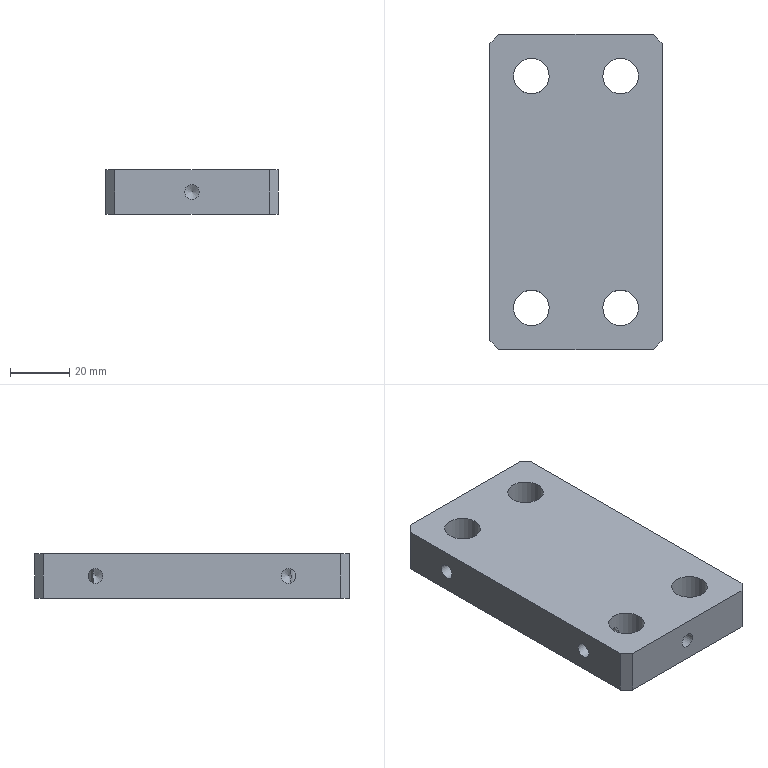Part | NX | features BREP 1 | 1 solid | 20 faces | box 58 x 106 x 15 mm | volume 84312 mm3 | plane 10 | cylinder 7 | cone 3 | commonest cylinder face diameters 12 x4 5 x3
STEP:
#1=CARTESIAN_POINT('',(-29.,50.,15.));
#2=VERTEX_POINT('',#1);
#3=CARTESIAN_POINT('',(-29.,-50.,15.));
#4=VERTEX_POINT('',#3);
#5=CARTESIAN_POINT('',(-29.,0.,15.));
#6=DIRECTION('',(0.,-1.,0.));
#7=VECTOR('',#6,1000.);
#8=LINE('',#5,#7);
#9=EDGE_CURVE('',#2,#4,#8,.T.);
#10=ORIENTED_EDGE('',*,*,#9,.T.);
#11=CARTESIAN_POINT('',(-26.,-53.,15.));
#12=VERTEX_POINT('',#11);
#13=CARTESIAN_POINT('',(-29.,-50.,15.));
#14=DIRECTION('',(0.7071,-0.7071,0.));
#15=VECTOR('',#14,1000.);
#16=LINE('',#13,#15);
#17=EDGE_CURVE('',#4,#12,#16,.T.);
#18=ORIENTED_EDGE('',*,*,#17,.T.);
#19=CARTESIAN_POINT('',(26.,-53.,15.));
#20=VERTEX_POINT('',#19);
#21=CARTESIAN_POINT('',(0.,-53.,15.));
#22=DIRECTION('',(1.,0.,0.));
#23=VECTOR('',#22,1000.);
#24=LINE('',#21,#23);
#25=EDGE_CURVE('',#12,#20,#24,.T.);
#26=ORIENTED_EDGE('',*,*,#25,.T.);
#27=CARTESIAN_POINT('',(29.,-50.,15.));
#28=VERTEX_POINT('',#27);
#29=CARTESIAN_POINT('',(26.,-53.,15.));
#30=DIRECTION('',(0.7071,0.7071,0.));
#31=VECTOR('',#30,1000.);
#32=LINE('',#29,#31);
#33=EDGE_CURVE('',#20,#28,#32,.T.);
#34=ORIENTED_EDGE('',*,*,#33,.T.);
#35=CARTESIAN_POINT('',(29.,50.,15.));
#36=VERTEX_POINT('',#35);
#37=CARTESIAN_POINT('',(29.,0.,15.));
#38=DIRECTION('',(0.,1.,0.));
#39=VECTOR('',#38,1000.);
#40=LINE('',#37,#39);
#41=EDGE_CURVE('',#28,#36,#40,.T.);
#42=ORIENTED_EDGE('',*,*,#41,.T.);
#43=CARTESIAN_POINT('',(26.,53.,15.));
#44=VERTEX_POINT('',#43);
#45=CARTESIAN_POINT('',(29.,50.,15.));
#46=DIRECTION('',(-0.7071,0.7071,0.));
#47=VECTOR('',#46,1000.);
#48=LINE('',#45,#47);
#49=EDGE_CURVE('',#36,#44,#48,.T.);
#50=ORIENTED_EDGE('',*,*,#49,.T.);
#51=CARTESIAN_POINT('',(-26.,53.,15.));
#52=VERTEX_POINT('',#51);
#53=CARTESIAN_POINT('',(0.,53.,15.));
#54=DIRECTION('',(-1.,0.,0.));
#55=VECTOR('',#54,1000.);
#56=LINE('',#53,#55);
#57=EDGE_CURVE('',#44,#52,#56,.T.);
#58=ORIENTED_EDGE('',*,*,#57,.T.);
#59=CARTESIAN_POINT('',(-26.,53.,15.));
#60=DIRECTION('',(-0.7071,-0.7071,0.));
#61=VECTOR('',#60,1000.);
#62=LINE('',#59,#61);
#63=EDGE_CURVE('',#52,#2,#62,.T.);
#64=ORIENTED_EDGE('',*,*,#63,.T.);
#65=EDGE_LOOP('',(#10,#18,#26,#34,#42,#50,#58,#64));
#66=FACE_BOUND('',#65,.T.);
#67=CARTESIAN_POINT('',(9.,-39.,15.));
#68=VERTEX_POINT('',#67);
#69=CARTESIAN_POINT('',(15.,-39.,15.));
#70=DIRECTION('',(0.,0.,-1.));
#71=DIRECTION('',(-1.,0.,0.));
#72=AXIS2_PLACEMENT_3D('',#69,#70,#71);
#73=CIRCLE('',#72,6.);
#74=EDGE_CURVE('',#68,#68,#73,.T.);
#75=ORIENTED_EDGE('',*,*,#74,.T.);
#76=EDGE_LOOP('',(#75));
#77=FACE_BOUND('',#76,.T.);
#78=CARTESIAN_POINT('',(-21.,-39.,15.));
#79=VERTEX_POINT('',#78);
#80=CARTESIAN_POINT('',(-15.,-39.,15.));
#81=DIRECTION('',(0.,0.,-1.));
#82=DIRECTION('',(-1.,0.,0.));
#83=AXIS2_PLACEMENT_3D('',#80,#81,#82);
#84=CIRCLE('',#83,6.);
#85=EDGE_CURVE('',#79,#79,#84,.T.);
#86=ORIENTED_EDGE('',*,*,#85,.T.);
#87=EDGE_LOOP('',(#86));
#88=FACE_BOUND('',#87,.T.);
#89=CARTESIAN_POINT('',(-21.,39.,15.));
#90=VERTEX_POINT('',#89);
#91=CARTESIAN_POINT('',(-15.,39.,15.));
#92=DIRECTION('',(0.,0.,-1.));
#93=DIRECTION('',(-1.,0.,0.));
#94=AXIS2_PLACEMENT_3D('',#91,#92,#93);
#95=CIRCLE('',#94,6.);
#96=EDGE_CURVE('',#90,#90,#95,.T.);
#97=ORIENTED_EDGE('',*,*,#96,.T.);
#98=EDGE_LOOP('',(#97));
#99=FACE_BOUND('',#98,.T.);
#100=CARTESIAN_POINT('',(9.,39.,15.));
#101=VERTEX_POINT('',#100);
#102=CARTESIAN_POINT('',(15.,39.,15.));
#103=DIRECTION('',(0.,0.,-1.));
#104=DIRECTION('',(-1.,0.,0.));
#105=AXIS2_PLACEMENT_3D('',#102,#103,#104);
#106=CIRCLE('',#105,6.);
#107=EDGE_CURVE('',#101,#101,#106,.T.);
#108=ORIENTED_EDGE('',*,*,#107,.T.);
#109=EDGE_LOOP('',(#108));
#110=FACE_BOUND('',#109,.T.);
#111=CARTESIAN_POINT('',(0.,0.,15.));
#112=DIRECTION('',(0.,0.,1.));
#113=DIRECTION('',(-1.,0.,0.));
#114=AXIS2_PLACEMENT_3D('',#111,#112,#113);
#115=PLANE('',#114);
#116=ADVANCED_FACE('',(#66,#77,#88,#99,#110),#115,.T.);
#117=CARTESIAN_POINT('',(-29.,-50.,0.));
#118=VERTEX_POINT('',#117);
#119=CARTESIAN_POINT('',(-29.,-50.,15.));
#120=DIRECTION('',(0.,0.,1.));
#121=VECTOR('',#120,1000.);
#122=LINE('',#119,#121);
#123=EDGE_CURVE('',#118,#4,#122,.T.);
#124=ORIENTED_EDGE('',*,*,#123,.F.);
#125=CARTESIAN_POINT('',(-26.,-53.,0.));
#126=VERTEX_POINT('',#125);
#127=CARTESIAN_POINT('',(-26.,-53.,0.));
#128=DIRECTION('',(-0.7071,0.7071,0.));
#129=VECTOR('',#128,1000.);
#130=LINE('',#127,#129);
#131=EDGE_CURVE('',#126,#118,#130,.T.);
#132=ORIENTED_EDGE('',*,*,#131,.F.);
#133=CARTESIAN_POINT('',(-26.,-53.,15.));
#134=DIRECTION('',(0.,0.,-1.));
#135=VECTOR('',#134,1000.);
#136=LINE('',#133,#135);
#137=EDGE_CURVE('',#12,#126,#136,.T.);
#138=ORIENTED_EDGE('',*,*,#137,.F.);
#139=ORIENTED_EDGE('',*,*,#17,.F.);
#140=EDGE_LOOP('',(#124,#132,#138,#139));
#141=FACE_BOUND('',#140,.T.);
#142=CARTESIAN_POINT('',(-26.,-53.,15.));
#143=DIRECTION('',(0.7071,0.7071,0.));
#144=DIRECTION('',(0.7071,-0.7071,0.));
#145=AXIS2_PLACEMENT_3D('',#142,#143,#144);
#146=PLANE('',#145);
#147=ADVANCED_FACE('',(#141),#146,.F.);
#148=ORIENTED_EDGE('',*,*,#123,.T.);
#149=ORIENTED_EDGE('',*,*,#9,.F.);
#150=CARTESIAN_POINT('',(-29.,50.,0.));
#151=VERTEX_POINT('',#150);
#152=CARTESIAN_POINT('',(-29.,50.,15.));
#153=DIRECTION('',(0.,0.,1.));
#154=VECTOR('',#153,1000.);
#155=LINE('',#152,#154);
#156=EDGE_CURVE('',#151,#2,#155,.T.);
#157=ORIENTED_EDGE('',*,*,#156,.F.);
#158=CARTESIAN_POINT('',(-29.,53.,0.));
#159=DIRECTION('',(0.,1.,0.));
#160=VECTOR('',#159,1000.);
#161=LINE('',#158,#160);
#162=EDGE_CURVE('',#118,#151,#161,.T.);
#163=ORIENTED_EDGE('',*,*,#162,.F.);
#164=EDGE_LOOP('',(#148,#149,#157,#163));
#165=FACE_BOUND('',#164,.T.);
#166=CARTESIAN_POINT('',(-29.,32.5,10.));
#167=VERTEX_POINT('',#166);
#168=CARTESIAN_POINT('',(-29.,32.5,7.5));
#169=DIRECTION('',(-1.,0.,0.));
#170=DIRECTION('',(0.,0.,1.));
#171=AXIS2_PLACEMENT_3D('',#168,#169,#170);
#172=CIRCLE('',#171,2.5);
#173=EDGE_CURVE('',#167,#167,#172,.T.);
#174=ORIENTED_EDGE('',*,*,#173,.F.);
#175=EDGE_LOOP('',(#174));
#176=FACE_BOUND('',#175,.T.);
#177=CARTESIAN_POINT('',(-29.,-32.5,10.));
#178=VERTEX_POINT('',#177);
#179=CARTESIAN_POINT('',(-29.,-32.5,7.5));
#180=DIRECTION('',(-1.,0.,0.));
#181=DIRECTION('',(0.,0.,1.));
#182=AXIS2_PLACEMENT_3D('',#179,#180,#181);
#183=CIRCLE('',#182,2.5);
#184=EDGE_CURVE('',#178,#178,#183,.T.);
#185=ORIENTED_EDGE('',*,*,#184,.F.);
#186=EDGE_LOOP('',(#185));
#187=FACE_BOUND('',#186,.T.);
#188=CARTESIAN_POINT('',(-29.,53.,15.));
#189=DIRECTION('',(1.,0.,0.));
#190=DIRECTION('',(0.,-1.,0.));
#191=AXIS2_PLACEMENT_3D('',#188,#189,#190);
#192=PLANE('',#191);
#193=ADVANCED_FACE('',(#165,#176,#187),#192,.F.);
#194=CARTESIAN_POINT('',(-26.,53.,0.));
#195=VERTEX_POINT('',#194);
#196=CARTESIAN_POINT('',(-26.,53.,15.));
#197=DIRECTION('',(0.,0.,1.));
#198=VECTOR('',#197,1000.);
#199=LINE('',#196,#198);
#200=EDGE_CURVE('',#195,#52,#199,.T.);
#201=ORIENTED_EDGE('',*,*,#200,.F.);
#202=CARTESIAN_POINT('',(-29.,50.,0.));
#203=DIRECTION('',(0.7071,0.7071,0.));
#204=VECTOR('',#203,1000.);
#205=LINE('',#202,#204);
#206=EDGE_CURVE('',#151,#195,#205,.T.);
#207=ORIENTED_EDGE('',*,*,#206,.F.);
#208=ORIENTED_EDGE('',*,*,#156,.T.);
#209=ORIENTED_EDGE('',*,*,#63,.F.);
#210=EDGE_LOOP('',(#201,#207,#208,#209));
#211=FACE_BOUND('',#210,.T.);
#212=CARTESIAN_POINT('',(-29.,50.,15.));
#213=DIRECTION('',(0.7071,-0.7071,0.));
#214=DIRECTION('',(-0.7071,-0.7071,0.));
#215=AXIS2_PLACEMENT_3D('',#212,#213,#214);
#216=PLANE('',#215);
#217=ADVANCED_FACE('',(#211),#216,.F.);
#218=CARTESIAN_POINT('',(26.,53.,0.));
#219=VERTEX_POINT('',#218);
#220=CARTESIAN_POINT('',(26.,53.,15.));
#221=DIRECTION('',(0.,0.,1.));
#222=VECTOR('',#221,1000.);
#223=LINE('',#220,#222);
#224=EDGE_CURVE('',#219,#44,#223,.T.);
#225=ORIENTED_EDGE('',*,*,#224,.F.);
#226=CARTESIAN_POINT('',(-29.,53.,0.));
#227=DIRECTION('',(1.,0.,0.));
#228=VECTOR('',#227,1000.);
#229=LINE('',#226,#228);
#230=EDGE_CURVE('',#195,#219,#229,.T.);
#231=ORIENTED_EDGE('',*,*,#230,.F.);
#232=ORIENTED_EDGE('',*,*,#200,.T.);
#233=ORIENTED_EDGE('',*,*,#57,.F.);
#234=EDGE_LOOP('',(#225,#231,#232,#233));
#235=FACE_BOUND('',#234,.T.);
#236=CARTESIAN_POINT('',(-29.,53.,15.));
#237=DIRECTION('',(0.,-1.,0.));
#238=DIRECTION('',(0.,0.,1.));
#239=AXIS2_PLACEMENT_3D('',#236,#237,#238);
#240=PLANE('',#239);
#241=ADVANCED_FACE('',(#235),#240,.F.);
#242=CARTESIAN_POINT('',(29.,50.,0.));
#243=VERTEX_POINT('',#242);
#244=CARTESIAN_POINT('',(29.,50.,15.));
#245=DIRECTION('',(0.,0.,1.));
#246=VECTOR('',#245,1000.);
#247=LINE('',#244,#246);
#248=EDGE_CURVE('',#243,#36,#247,.T.);
#249=ORIENTED_EDGE('',*,*,#248,.F.);
#250=CARTESIAN_POINT('',(26.,53.,0.));
#251=DIRECTION('',(0.7071,-0.7071,0.));
#252=VECTOR('',#251,1000.);
#253=LINE('',#250,#252);
#254=EDGE_CURVE('',#219,#243,#253,.T.);
#255=ORIENTED_EDGE('',*,*,#254,.F.);
#256=ORIENTED_EDGE('',*,*,#224,.T.);
#257=ORIENTED_EDGE('',*,*,#49,.F.);
#258=EDGE_LOOP('',(#249,#255,#256,#257));
#259=FACE_BOUND('',#258,.T.);
#260=CARTESIAN_POINT('',(26.,53.,15.));
#261=DIRECTION('',(-0.7071,-0.7071,0.));
#262=DIRECTION('',(-0.7071,0.7071,0.));
#263=AXIS2_PLACEMENT_3D('',#260,#261,#262);
#264=PLANE('',#263);
#265=ADVANCED_FACE('',(#259),#264,.F.);
#266=CARTESIAN_POINT('',(29.,-50.,0.));
#267=VERTEX_POINT('',#266);
#268=CARTESIAN_POINT('',(29.,-50.,15.));
#269=DIRECTION('',(0.,0.,1.));
#270=VECTOR('',#269,1000.);
#271=LINE('',#268,#270);
#272=EDGE_CURVE('',#267,#28,#271,.T.);
#273=ORIENTED_EDGE('',*,*,#272,.F.);
#274=CARTESIAN_POINT('',(29.,53.,0.));
#275=DIRECTION('',(0.,-1.,0.));
#276=VECTOR('',#275,1000.);
#277=LINE('',#274,#276);
#278=EDGE_CURVE('',#243,#267,#277,.T.);
#279=ORIENTED_EDGE('',*,*,#278,.F.);
#280=ORIENTED_EDGE('',*,*,#248,.T.);
#281=ORIENTED_EDGE('',*,*,#41,.F.);
#282=EDGE_LOOP('',(#273,#279,#280,#281));
#283=FACE_BOUND('',#282,.T.);
#284=CARTESIAN_POINT('',(29.,53.,15.));
#285=DIRECTION('',(-1.,0.,0.));
#286=DIRECTION('',(0.,1.,0.));
#287=AXIS2_PLACEMENT_3D('',#284,#285,#286);
#288=PLANE('',#287);
#289=ADVANCED_FACE('',(#283),#288,.F.);
#290=CARTESIAN_POINT('',(26.,-53.,0.));
#291=VERTEX_POINT('',#290);
#292=CARTESIAN_POINT('',(26.,-53.,15.));
#293=DIRECTION('',(0.,0.,1.));
#294=VECTOR('',#293,1000.);
#295=LINE('',#292,#294);
#296=EDGE_CURVE('',#291,#20,#295,.T.);
#297=ORIENTED_EDGE('',*,*,#296,.F.);
#298=CARTESIAN_POINT('',(29.,-50.,0.));
#299=DIRECTION('',(-0.7071,-0.7071,0.));
#300=VECTOR('',#299,1000.);
#301=LINE('',#298,#300);
#302=EDGE_CURVE('',#267,#291,#301,.T.);
#303=ORIENTED_EDGE('',*,*,#302,.F.);
#304=ORIENTED_EDGE('',*,*,#272,.T.);
#305=ORIENTED_EDGE('',*,*,#33,.F.);
#306=EDGE_LOOP('',(#297,#303,#304,#305));
#307=FACE_BOUND('',#306,.T.);
#308=CARTESIAN_POINT('',(29.,-50.,15.));
#309=DIRECTION('',(-0.7071,0.7071,0.));
#310=DIRECTION('',(0.7071,0.7071,0.));
#311=AXIS2_PLACEMENT_3D('',#308,#309,#310);
#312=PLANE('',#311);
#313=ADVANCED_FACE('',(#307),#312,.F.);
#314=ORIENTED_EDGE('',*,*,#296,.T.);
#315=ORIENTED_EDGE('',*,*,#25,.F.);
#316=ORIENTED_EDGE('',*,*,#137,.T.);
#317=CARTESIAN_POINT('',(-29.,-53.,0.));
#318=DIRECTION('',(-1.,0.,0.));
#319=VECTOR('',#318,1000.);
#320=LINE('',#317,#319);
#321=EDGE_CURVE('',#291,#126,#320,.T.);
#322=ORIENTED_EDGE('',*,*,#321,.F.);
#323=EDGE_LOOP('',(#314,#315,#316,#322));
#324=FACE_BOUND('',#323,.T.);
#325=CARTESIAN_POINT('',(0.,-53.,5.));
#326=VERTEX_POINT('',#325);
#327=CARTESIAN_POINT('',(0.,-53.,7.5));
#328=DIRECTION('',(0.,-1.,0.));
#329=DIRECTION('',(0.,0.,-1.));
#330=AXIS2_PLACEMENT_3D('',#327,#328,#329);
#331=CIRCLE('',#330,2.5);
#332=EDGE_CURVE('',#326,#326,#331,.T.);
#333=ORIENTED_EDGE('',*,*,#332,.F.);
#334=EDGE_LOOP('',(#333));
#335=FACE_BOUND('',#334,.T.);
#336=CARTESIAN_POINT('',(-29.,-53.,15.));
#337=DIRECTION('',(0.,1.,0.));
#338=DIRECTION('',(0.,0.,-1.));
#339=AXIS2_PLACEMENT_3D('',#336,#337,#338);
#340=PLANE('',#339);
#341=ADVANCED_FACE('',(#324,#335),#340,.F.);
#342=CARTESIAN_POINT('',(9.,-39.,0.));
#343=VERTEX_POINT('',#342);
#344=CARTESIAN_POINT('',(15.,-39.,0.));
#345=DIRECTION('',(0.,0.,1.));
#346=DIRECTION('',(-1.,0.,0.));
#347=AXIS2_PLACEMENT_3D('',#344,#345,#346);
#348=CIRCLE('',#347,6.);
#349=EDGE_CURVE('',#343,#343,#348,.T.);
#350=ORIENTED_EDGE('',*,*,#349,.F.);
#351=EDGE_LOOP('',(#350));
#352=FACE_BOUND('',#351,.T.);
#353=ORIENTED_EDGE('',*,*,#74,.F.);
#354=EDGE_LOOP('',(#353));
#355=FACE_BOUND('',#354,.T.);
#356=CARTESIAN_POINT('',(15.,-39.,0.));
#357=DIRECTION('',(0.,0.,-1.));
#358=DIRECTION('',(1.,0.,0.));
#359=AXIS2_PLACEMENT_3D('',#356,#357,#358);
#360=CYLINDRICAL_SURFACE('',#359,6.);
#361=ADVANCED_FACE('',(#352,#355),#360,.F.);
#362=CARTESIAN_POINT('',(-21.,-39.,0.));
#363=VERTEX_POINT('',#362);
#364=CARTESIAN_POINT('',(-15.,-39.,0.));
#365=DIRECTION('',(0.,0.,1.));
#366=DIRECTION('',(-1.,0.,0.));
#367=AXIS2_PLACEMENT_3D('',#364,#365,#366);
#368=CIRCLE('',#367,6.);
#369=EDGE_CURVE('',#363,#363,#368,.T.);
#370=ORIENTED_EDGE('',*,*,#369,.F.);
#371=EDGE_LOOP('',(#370));
#372=FACE_BOUND('',#371,.T.);
#373=ORIENTED_EDGE('',*,*,#85,.F.);
#374=EDGE_LOOP('',(#373));
#375=FACE_BOUND('',#374,.T.);
#376=CARTESIAN_POINT('',(-14.,-33.084,9.931));
#377=VERTEX_POINT('',#376);
#378=CARTESIAN_POINT('',(-14.,-33.084,5.069));
#379=VERTEX_POINT('',#378);
#380=CARTESIAN_POINT('',(-14.,-33.084,9.931));
#381=CARTESIAN_POINT('',(-14.598,-32.983,9.955));
#382=CARTESIAN_POINT('',(-15.805,-32.966,9.957));
#383=CARTESIAN_POINT('',(-17.547,-33.461,9.846));
#384=CARTESIAN_POINT('',(-19.042,-34.481,9.275));
#385=CARTESIAN_POINT('',(-19.685,-35.257,7.513));
#386=CARTESIAN_POINT('',(-19.053,-34.492,5.735));
#387=CARTESIAN_POINT('',(-17.568,-33.471,5.157));
#388=CARTESIAN_POINT('',(-15.82,-32.966,5.043));
#389=CARTESIAN_POINT('',(-14.598,-32.983,5.045));
#390=CARTESIAN_POINT('',(-14.,-33.084,5.069));
#391=B_SPLINE_CURVE_WITH_KNOTS('',3,(#380,#381,#382,#383,#384,#385,#386,#387,#388,#389,#390),.UNSPECIFIED.,.F.,.F.,(4,1,1,1,1,1,1,1,4),(0.,0.001794,0.003588,0.005381,0.007175,0.008969,0.01076,0.01256,0.01435),.UNSPECIFIED.);
#392=EDGE_CURVE('',#377,#379,#391,.T.);
#393=ORIENTED_EDGE('',*,*,#392,.F.);
#394=CARTESIAN_POINT('',(-14.,-33.084,5.069));
#395=CARTESIAN_POINT('',(-13.78,-33.121,5.455));
#396=CARTESIAN_POINT('',(-13.353,-33.219,6.213));
#397=CARTESIAN_POINT('',(-12.829,-33.404,7.503));
#398=CARTESIAN_POINT('',(-13.355,-33.218,8.789));
#399=CARTESIAN_POINT('',(-13.781,-33.121,9.546));
#400=CARTESIAN_POINT('',(-14.,-33.084,9.931));
#401=B_SPLINE_CURVE_WITH_KNOTS('',3,(#394,#395,#396,#397,#398,#399,#400),.UNSPECIFIED.,.F.,.F.,(4,1,1,1,4),(0.,0.001335,0.002669,0.004004,0.005339),.UNSPECIFIED.);
#402=EDGE_CURVE('',#379,#377,#401,.T.);
#403=ORIENTED_EDGE('',*,*,#402,.F.);
#404=EDGE_LOOP('',(#393,#403));
#405=FACE_BOUND('',#404,.T.);
#406=CARTESIAN_POINT('',(-15.,-39.,0.));
#407=DIRECTION('',(0.,0.,-1.));
#408=DIRECTION('',(1.,0.,0.));
#409=AXIS2_PLACEMENT_3D('',#406,#407,#408);
#410=CYLINDRICAL_SURFACE('',#409,6.);
#411=ADVANCED_FACE('',(#372,#375,#405),#410,.F.);
#412=CARTESIAN_POINT('',(-21.,39.,0.));
#413=VERTEX_POINT('',#412);
#414=CARTESIAN_POINT('',(-15.,39.,0.));
#415=DIRECTION('',(0.,0.,1.));
#416=DIRECTION('',(-1.,0.,0.));
#417=AXIS2_PLACEMENT_3D('',#414,#415,#416);
#418=CIRCLE('',#417,6.);
#419=EDGE_CURVE('',#413,#413,#418,.T.);
#420=ORIENTED_EDGE('',*,*,#419,.F.);
#421=EDGE_LOOP('',(#420));
#422=FACE_BOUND('',#421,.T.);
#423=ORIENTED_EDGE('',*,*,#96,.F.);
#424=EDGE_LOOP('',(#423));
#425=FACE_BOUND('',#424,.T.);
#426=CARTESIAN_POINT('',(-14.,33.084,5.069));
#427=VERTEX_POINT('',#426);
#428=CARTESIAN_POINT('',(-14.,33.084,9.931));
#429=VERTEX_POINT('',#428);
#430=CARTESIAN_POINT('',(-14.,33.084,5.069));
#431=CARTESIAN_POINT('',(-14.598,32.983,5.045));
#432=CARTESIAN_POINT('',(-15.805,32.966,5.043));
#433=CARTESIAN_POINT('',(-17.547,33.461,5.154));
#434=CARTESIAN_POINT('',(-19.042,34.481,5.725));
#435=CARTESIAN_POINT('',(-19.685,35.257,7.487));
#436=CARTESIAN_POINT('',(-19.053,34.492,9.265));
#437=CARTESIAN_POINT('',(-17.568,33.471,9.843));
#438=CARTESIAN_POINT('',(-15.82,32.966,9.957));
#439=CARTESIAN_POINT('',(-14.598,32.983,9.955));
#440=CARTESIAN_POINT('',(-14.,33.084,9.931));
#441=B_SPLINE_CURVE_WITH_KNOTS('',3,(#430,#431,#432,#433,#434,#435,#436,#437,#438,#439,#440),.UNSPECIFIED.,.F.,.F.,(4,1,1,1,1,1,1,1,4),(0.,0.001794,0.003588,0.005381,0.007175,0.008969,0.01076,0.01256,0.01435),.UNSPECIFIED.);
#442=EDGE_CURVE('',#427,#429,#441,.T.);
#443=ORIENTED_EDGE('',*,*,#442,.F.);
#444=CARTESIAN_POINT('',(-14.,33.084,9.931));
#445=CARTESIAN_POINT('',(-13.78,33.121,9.545));
#446=CARTESIAN_POINT('',(-13.353,33.219,8.787));
#447=CARTESIAN_POINT('',(-12.829,33.404,7.497));
#448=CARTESIAN_POINT('',(-13.355,33.218,6.211));
#449=CARTESIAN_POINT('',(-13.781,33.121,5.454));
#450=CARTESIAN_POINT('',(-14.,33.084,5.069));
#451=B_SPLINE_CURVE_WITH_KNOTS('',3,(#444,#445,#446,#447,#448,#449,#450),.UNSPECIFIED.,.F.,.F.,(4,1,1,1,4),(0.,0.001335,0.002669,0.004004,0.005339),.UNSPECIFIED.);
#452=EDGE_CURVE('',#429,#427,#451,.T.);
#453=ORIENTED_EDGE('',*,*,#452,.F.);
#454=EDGE_LOOP('',(#443,#453));
#455=FACE_BOUND('',#454,.T.);
#456=CARTESIAN_POINT('',(-15.,39.,0.));
#457=DIRECTION('',(0.,0.,-1.));
#458=DIRECTION('',(1.,0.,0.));
#459=AXIS2_PLACEMENT_3D('',#456,#457,#458);
#460=CYLINDRICAL_SURFACE('',#459,6.);
#461=ADVANCED_FACE('',(#422,#425,#455),#460,.F.);
#462=CARTESIAN_POINT('',(9.,39.,0.));
#463=VERTEX_POINT('',#462);
#464=CARTESIAN_POINT('',(15.,39.,0.));
#465=DIRECTION('',(0.,0.,1.));
#466=DIRECTION('',(-1.,0.,0.));
#467=AXIS2_PLACEMENT_3D('',#464,#465,#466);
#468=CIRCLE('',#467,6.);
#469=EDGE_CURVE('',#463,#463,#468,.T.);
#470=ORIENTED_EDGE('',*,*,#469,.F.);
#471=EDGE_LOOP('',(#470));
#472=FACE_BOUND('',#471,.T.);
#473=ORIENTED_EDGE('',*,*,#107,.F.);
#474=EDGE_LOOP('',(#473));
#475=FACE_BOUND('',#474,.T.);
#476=CARTESIAN_POINT('',(15.,39.,0.));
#477=DIRECTION('',(0.,0.,-1.));
#478=DIRECTION('',(1.,0.,0.));
#479=AXIS2_PLACEMENT_3D('',#476,#477,#478);
#480=CYLINDRICAL_SURFACE('',#479,6.);
#481=ADVANCED_FACE('',(#472,#475),#480,.F.);
#482=ORIENTED_EDGE('',*,*,#302,.T.);
#483=ORIENTED_EDGE('',*,*,#321,.T.);
#484=ORIENTED_EDGE('',*,*,#131,.T.);
#485=ORIENTED_EDGE('',*,*,#162,.T.);
#486=ORIENTED_EDGE('',*,*,#206,.T.);
#487=ORIENTED_EDGE('',*,*,#230,.T.);
#488=ORIENTED_EDGE('',*,*,#254,.T.);
#489=ORIENTED_EDGE('',*,*,#278,.T.);
#490=EDGE_LOOP('',(#482,#483,#484,#485,#486,#487,#488,#489));
#491=FACE_BOUND('',#490,.T.);
#492=ORIENTED_EDGE('',*,*,#349,.T.);
#493=EDGE_LOOP('',(#492));
#494=FACE_BOUND('',#493,.T.);
#495=ORIENTED_EDGE('',*,*,#369,.T.);
#496=EDGE_LOOP('',(#495));
#497=FACE_BOUND('',#496,.T.);
#498=ORIENTED_EDGE('',*,*,#419,.T.);
#499=EDGE_LOOP('',(#498));
#500=FACE_BOUND('',#499,.T.);
#501=ORIENTED_EDGE('',*,*,#469,.T.);
#502=EDGE_LOOP('',(#501));
#503=FACE_BOUND('',#502,.T.);
#504=CARTESIAN_POINT('',(0.,0.,0.));
#505=DIRECTION('',(0.,0.,1.));
#506=DIRECTION('',(-1.,0.,0.));
#507=AXIS2_PLACEMENT_3D('',#504,#505,#506);
#508=PLANE('',#507);
#509=ADVANCED_FACE('',(#491,#494,#497,#500,#503),#508,.F.);
#510=ORIENTED_EDGE('',*,*,#442,.T.);
#511=CARTESIAN_POINT('',(-14.,32.5,7.5));
#512=DIRECTION('',(-1.,0.,0.));
#513=DIRECTION('',(0.,0.,1.));
#514=AXIS2_PLACEMENT_3D('',#511,#512,#513);
#515=CIRCLE('',#514,2.5);
#516=EDGE_CURVE('',#427,#429,#515,.T.);
#517=ORIENTED_EDGE('',*,*,#516,.F.);
#518=EDGE_LOOP('',(#510,#517));
#519=FACE_BOUND('',#518,.T.);
#520=ORIENTED_EDGE('',*,*,#173,.T.);
#521=EDGE_LOOP('',(#520));
#522=FACE_BOUND('',#521,.T.);
#523=CARTESIAN_POINT('',(-29.,32.5,7.5));
#524=DIRECTION('',(-1.,0.,0.));
#525=DIRECTION('',(0.,0.,-1.));
#526=AXIS2_PLACEMENT_3D('',#523,#524,#525);
#527=CYLINDRICAL_SURFACE('',#526,2.5);
#528=ADVANCED_FACE('',(#519,#522),#527,.F.);
#529=CARTESIAN_POINT('',(-14.,-32.5,7.5));
#530=DIRECTION('',(-1.,0.,0.));
#531=DIRECTION('',(0.,0.,1.));
#532=AXIS2_PLACEMENT_3D('',#529,#530,#531);
#533=CIRCLE('',#532,2.5);
#534=EDGE_CURVE('',#377,#379,#533,.T.);
#535=ORIENTED_EDGE('',*,*,#534,.F.);
#536=ORIENTED_EDGE('',*,*,#392,.T.);
#537=EDGE_LOOP('',(#535,#536));
#538=FACE_BOUND('',#537,.T.);
#539=ORIENTED_EDGE('',*,*,#184,.T.);
#540=EDGE_LOOP('',(#539));
#541=FACE_BOUND('',#540,.T.);
#542=CARTESIAN_POINT('',(-29.,-32.5,7.5));
#543=DIRECTION('',(-1.,0.,0.));
#544=DIRECTION('',(0.,0.,-1.));
#545=AXIS2_PLACEMENT_3D('',#542,#543,#544);
#546=CYLINDRICAL_SURFACE('',#545,2.5);
#547=ADVANCED_FACE('',(#538,#541),#546,.F.);
#548=CARTESIAN_POINT('',(0.,-38.,5.));
#549=VERTEX_POINT('',#548);
#550=CARTESIAN_POINT('',(0.,-38.,7.5));
#551=DIRECTION('',(0.,-1.,0.));
#552=DIRECTION('',(0.,0.,-1.));
#553=AXIS2_PLACEMENT_3D('',#550,#551,#552);
#554=CIRCLE('',#553,2.5);
#555=EDGE_CURVE('',#549,#549,#554,.T.);
#556=ORIENTED_EDGE('',*,*,#555,.F.);
#557=EDGE_LOOP('',(#556));
#558=FACE_BOUND('',#557,.T.);
#559=ORIENTED_EDGE('',*,*,#332,.T.);
#560=EDGE_LOOP('',(#559));
#561=FACE_BOUND('',#560,.T.);
#562=CARTESIAN_POINT('',(0.,-53.,7.5));
#563=DIRECTION('',(0.,-1.,0.));
#564=DIRECTION('',(0.,0.,1.));
#565=AXIS2_PLACEMENT_3D('',#562,#563,#564);
#566=CYLINDRICAL_SURFACE('',#565,2.5);
#567=ADVANCED_FACE('',(#558,#561),#566,.F.);
#568=ORIENTED_EDGE('',*,*,#534,.T.);
#569=ORIENTED_EDGE('',*,*,#402,.T.);
#570=EDGE_LOOP('',(#568,#569));
#571=FACE_BOUND('',#570,.T.);
#572=CARTESIAN_POINT('',(-14.,-32.5,7.5));
#573=DIRECTION('',(-1.,0.,0.));
#574=DIRECTION('',(0.,0.,-1.));
#575=AXIS2_PLACEMENT_3D('',#572,#573,#574);
#576=CONICAL_SURFACE('',#575,2.5,1.03);
#577=ADVANCED_FACE('',(#571),#576,.F.);
#578=ORIENTED_EDGE('',*,*,#516,.T.);
#579=ORIENTED_EDGE('',*,*,#452,.T.);
#580=EDGE_LOOP('',(#578,#579));
#581=FACE_BOUND('',#580,.T.);
#582=CARTESIAN_POINT('',(-14.,32.5,7.5));
#583=DIRECTION('',(-1.,0.,0.));
#584=DIRECTION('',(0.,0.,-1.));
#585=AXIS2_PLACEMENT_3D('',#582,#583,#584);
#586=CONICAL_SURFACE('',#585,2.5,1.03);
#587=ADVANCED_FACE('',(#581),#586,.F.);
#588=CARTESIAN_POINT('',(0.,-36.498,7.5));
#589=VERTEX_POINT('',#588);
#590=VERTEX_LOOP('',#589);
#591=FACE_BOUND('',#590,.T.);
#592=ORIENTED_EDGE('',*,*,#555,.T.);
#593=EDGE_LOOP('',(#592));
#594=FACE_BOUND('',#593,.T.);
#595=CARTESIAN_POINT('',(0.,-38.,7.5));
#596=DIRECTION('',(0.,-1.,0.));
#597=DIRECTION('',(0.,0.,1.));
#598=AXIS2_PLACEMENT_3D('',#595,#596,#597);
#599=CONICAL_SURFACE('',#598,2.5,1.03);
#600=ADVANCED_FACE('',(#591,#594),#599,.F.);
#601=CLOSED_SHELL('',(#116,#147,#193,#217,#241,#265,#289,#313,#341,#361,#411,#461,#481,#509,#528,#547,#567,#577,#587,#600));
#602=MANIFOLD_SOLID_BREP('',#601);
#603=(LENGTH_UNIT()NAMED_UNIT(*)SI_UNIT(.MILLI.,.METRE.));
#604=UNCERTAINTY_MEASURE_WITH_UNIT(LENGTH_MEASURE(0.0508),#603,'','');
#605=(NAMED_UNIT(*)PLANE_ANGLE_UNIT()SI_UNIT($,.RADIAN.));
#606=(NAMED_UNIT(*)SI_UNIT($,.STERADIAN.)SOLID_ANGLE_UNIT());
#607=(GEOMETRIC_REPRESENTATION_CONTEXT(3)GLOBAL_UNCERTAINTY_ASSIGNED_CONTEXT((#604))GLOBAL_UNIT_ASSIGNED_CONTEXT((#603,#605,#606))REPRESENTATION_CONTEXT('',''));
#608=ADVANCED_BREP_SHAPE_REPRESENTATION('',(#602),#607);